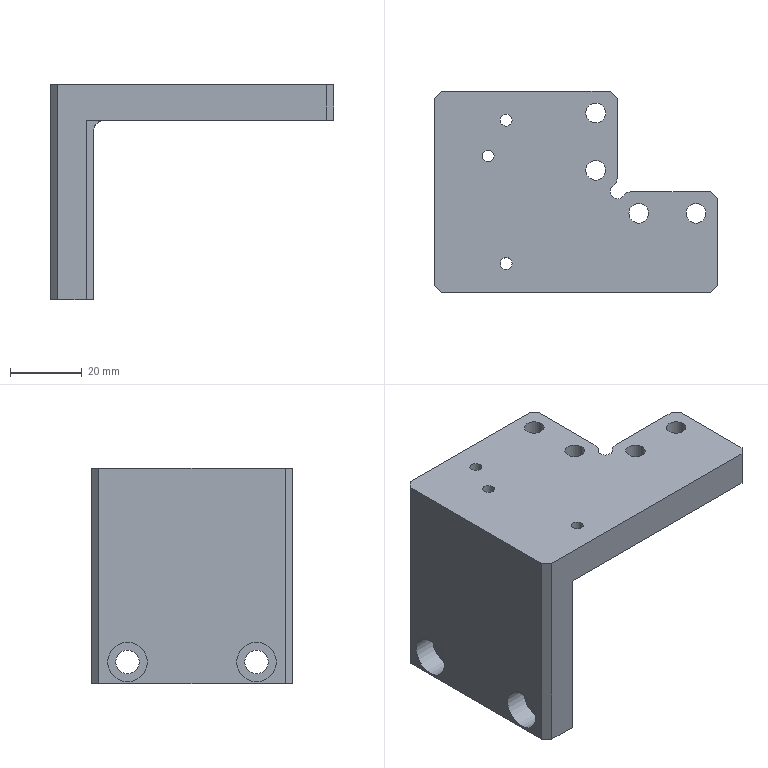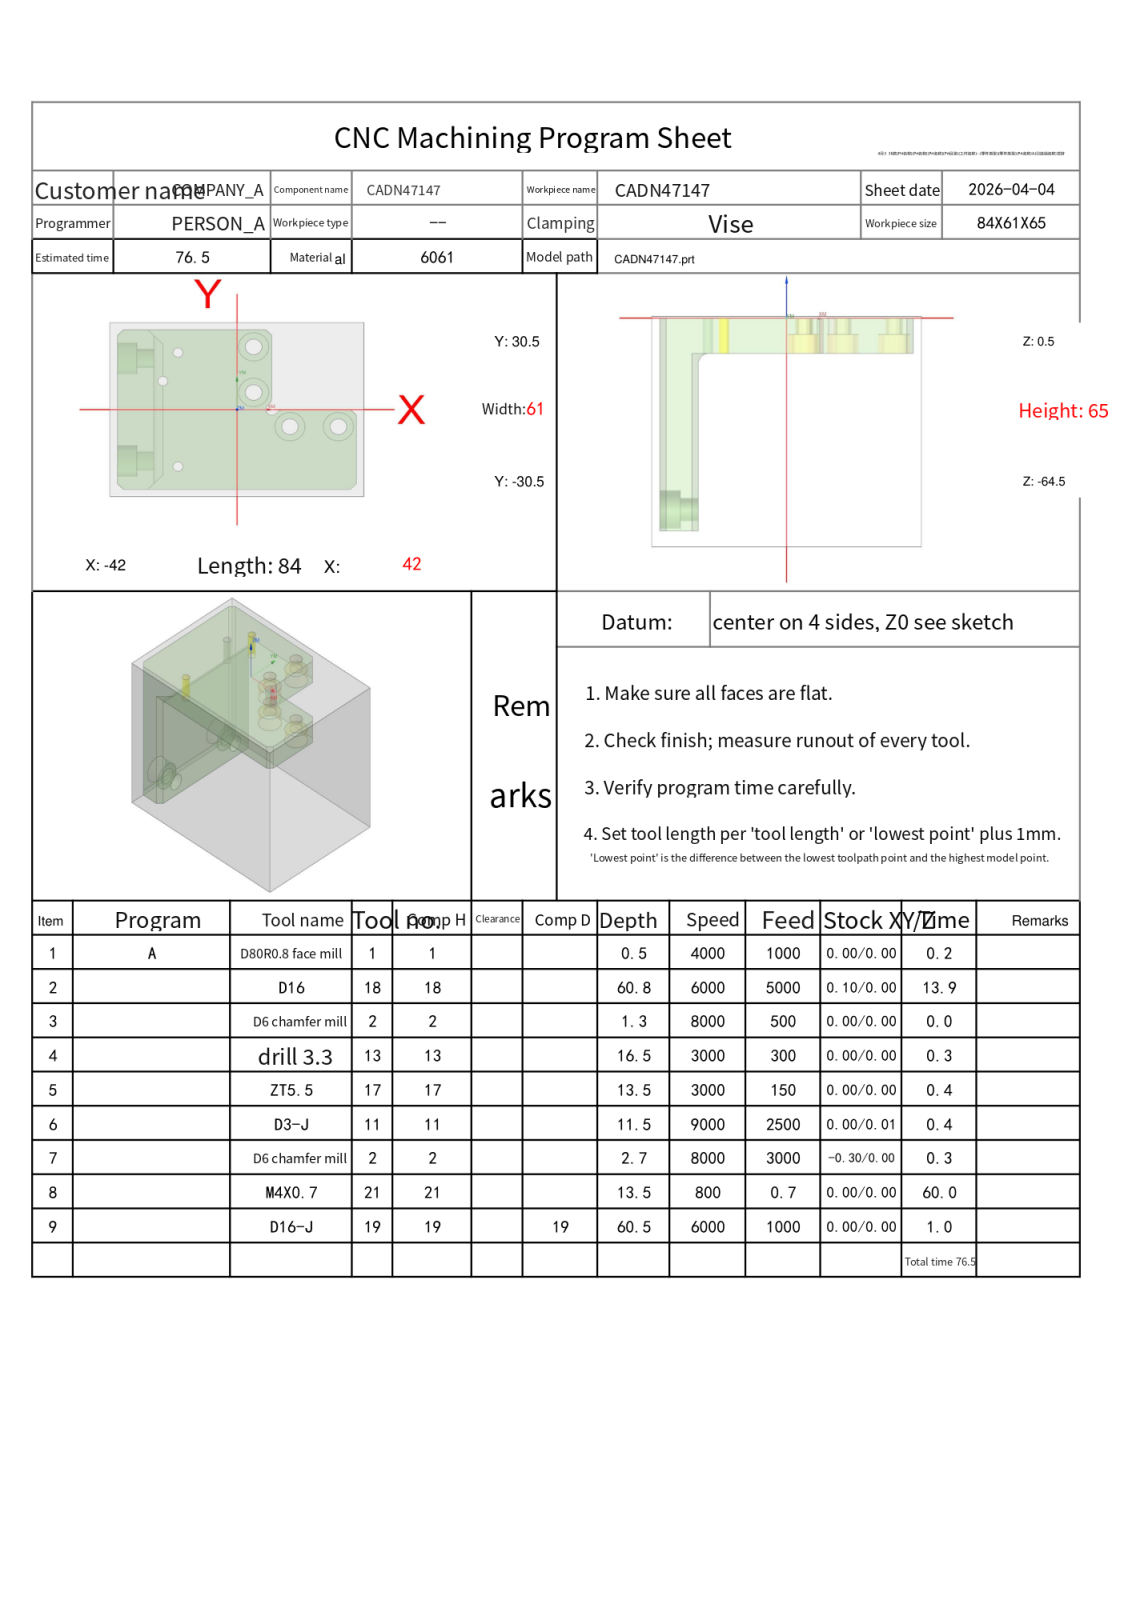NC program | NX | posted by the shop | part box 79 x 56 x 60 mm
Lines 35 to 1262 of 9053:
N2 T18 M06
(D16  D=16. R=0. H=18 ce=0.50 di=0.10)
G00 G90 G54 X61.191 Y31.1 M03 S6000
G43 H18 Z10.5
M08
Z.702
G01 Z-.498 F4000.
X54.
G03 X42.8 Y19.9 I0.0 J-11.2
G01 Y9.341
G02 X45.094 Y7.594 I-5.3 J-9.341
G01 X47.094 Y5.594
G02 X50. Y.258 I-7.594 J-7.594
G01 Y-7.414
X48.
Y-2.
G03 X45.51 Y4.01 I-8.5 J0.0
G01 X43.51 Y6.01
G03 X37.5 Y8.5 I-6.01 J-6.01
G01 X20.
Y26.
G03 X17.51 Y32.01 I-8.5 J0.0
G01 X15.51 Y34.01
G03 X9.5 Y36.5 I-6.01 J-6.01
G01 X-2.314
X-2.27 Y38.5
X11.758
G02 X17.094 Y35.594 I-2.258 J-10.5
G01 X19.094 Y33.594
G02 X20.841 Y31.3 I-7.594 J-7.594
G01 X42.
G02 X42.8 Y30.5 I0.0 J-.8
G01 Y11.9
G02 X41.2 Y10.3 I-1.6 J0.0
X40.385 Y10.523 I0.0 J1.6
G01 X32.009 Y15.477
G03 X31.195 Y15.7 I-.814 J-1.377
G01 X28.797
G02 X27.2 Y17.297 I.003 J1.6
G01 Y22.503
G02 X28.797 Y24.1 I1.6 J-.003
G01 X34.003
G02 X35.6 Y22.503 I-.003 J-1.6
G01 Y17.297
G02 X35.364 Y16.463 I-1.6 J.003
X35.04 Y16.084 I-1.364 J.837
G03 X33.099 Y12.263 I3.641 J-4.254
G01 X61.2
Z.702
G00 Z3.
G01 X61.191 Y31.1 F6000.
G00 Z.203
G01 Z-.997 F4000.
X54.
G03 X42.8 Y19.9 I0.0 J-11.2
G01 Y9.341
G02 X45.094 Y7.594 I-5.3 J-9.341
G01 X47.094 Y5.594
G02 X50. Y.258 I-7.594 J-7.594
G01 Y-7.414
X48.
Y-2.
G03 X45.51 Y4.01 I-8.5 J0.0
G01 X43.51 Y6.01
G03 X37.5 Y8.5 I-6.01 J-6.01
G01 X20.
Y10.74
Y26.
G03 X17.51 Y32.01 I-8.5 J0.0
G01 X15.51 Y34.01
G03 X9.5 Y36.5 I-6.01 J-6.01
G01 X-2.314
X-2.27 Y38.5
X11.758
G02 X17.094 Y35.594 I-2.258 J-10.5
G01 X19.094 Y33.594
G02 X20.841 Y31.3 I-7.594 J-7.594
G01 X42.
G02 X42.8 Y30.5 I0.0 J-.8
G01 Y11.9
G02 X41.2 Y10.3 I-1.6 J0.0
X40.385 Y10.523 I0.0 J1.6
G01 X32.009 Y15.477
G03 X31.195 Y15.7 I-.814 J-1.377
G01 X28.798
G02 X27.2 Y17.298 I.002 J1.6
G01 Y22.502
G02 X28.798 Y24.1 I1.6 J-.002
G01 X34.002
G02 X35.6 Y22.502 I-.002 J-1.6
G01 Y17.298
G02 X35.364 Y16.463 I-1.6 J.002
X35.04 Y16.084 I-1.364 J.837
G03 X33.099 Y12.263 I3.641 J-4.254
G01 X61.2
Z.203
G00 Z2.502
G01 X61.191 Y31.1 F6000.
G00 Z-.295
G01 Z-1.495 F4000.
X54.
G03 X42.8 Y19.9 I0.0 J-11.2
G01 Y9.341
G02 X45.094 Y7.594 I-5.3 J-9.341
G01 X47.094 Y5.594
G02 X50. Y.258 I-7.594 J-7.594
G01 Y-7.414
X48.
Y-2.
G03 X45.51 Y4.01 I-8.5 J0.0
G01 X43.51 Y6.01
G03 X37.5 Y8.5 I-6.01 J-6.01
G01 X20.
Y26.
G03 X17.51 Y32.01 I-8.5 J0.0
G01 X15.51 Y34.01
G03 X9.5 Y36.5 I-6.01 J-6.01
G01 X-2.314
X-2.27 Y38.5
X11.758
G02 X17.094 Y35.594 I-2.258 J-10.5
G01 X19.094 Y33.594
G02 X20.841 Y31.3 I-7.594 J-7.594
G01 X42.
G02 X42.8 Y30.5 I0.0 J-.8
G01 Y11.9
G02 X41.2 Y10.3 I-1.6 J0.0
X40.385 Y10.523 I0.0 J1.6
G01 X32.009 Y15.477
G03 X31.195 Y15.7 I-.814 J-1.377
G01 X28.797
G02 X27.2 Y17.297 I.003 J1.6
G01 Y22.503
G02 X28.797 Y24.1 I1.6 J-.003
G01 X34.003
G02 X35.6 Y22.503 I-.003 J-1.6
G01 Y17.297
G02 X35.364 Y16.463 I-1.6 J.003
X35.04 Y16.084 I-1.364 J.837
G03 X33.099 Y12.263 I3.641 J-4.254
G01 X61.2
Z-.295
G00 Z2.003
G01 X61.191 Y31.1 F6000.
G00 Z-.793
G01 Z-1.993 F4000.
X54.
G03 X42.8 Y19.9 I0.0 J-11.2
G01 Y9.341
G02 X45.094 Y7.594 I-5.3 J-9.341
G01 X47.094 Y5.594
G02 X50. Y.258 I-7.594 J-7.594
G01 Y-7.414
X48.
Y-2.
G03 X45.51 Y4.01 I-8.5 J0.0
G01 X43.51 Y6.01
G03 X37.5 Y8.5 I-6.01 J-6.01
G01 X20.
Y10.74
Y26.
G03 X17.51 Y32.01 I-8.5 J0.0
G01 X15.51 Y34.01
G03 X9.5 Y36.5 I-6.01 J-6.01
G01 X-2.314
X-2.27 Y38.5
X11.758
G02 X17.094 Y35.594 I-2.258 J-10.5
G01 X19.094 Y33.594
G02 X20.841 Y31.3 I-7.594 J-7.594
G01 X42.
G02 X42.8 Y30.5 I0.0 J-.8
G01 Y11.9
G02 X41.2 Y10.3 I-1.6 J0.0
X40.385 Y10.523 I0.0 J1.6
G01 X32.009 Y15.477
G03 X31.195 Y15.7 I-.814 J-1.377
G01 X28.798
G02 X27.2 Y17.298 I.002 J1.6
G01 Y22.502
G02 X28.798 Y24.1 I1.6 J-.002
G01 X34.002
G02 X35.6 Y22.502 I-.002 J-1.6
G01 Y17.298
G02 X35.364 Y16.463 I-1.6 J.002
X35.04 Y16.084 I-1.364 J.837
G03 X33.099 Y12.263 I3.641 J-4.254
G01 X61.2
Z-.793
G00 Z1.505
G01 X61.191 Y31.1 F6000.
G00 Z-1.292
G01 Z-2.492 F4000.
X54.
G03 X42.8 Y19.9 I0.0 J-11.2
G01 Y9.341
G02 X45.094 Y7.594 I-5.3 J-9.341
G01 X47.094 Y5.594
G02 X50. Y.258 I-7.594 J-7.594
G01 Y-7.414
X48.
Y-2.
G03 X45.51 Y4.01 I-8.5 J0.0
G01 X43.51 Y6.01
G03 X37.5 Y8.5 I-6.01 J-6.01
G01 X20.
Y26.
G03 X17.51 Y32.01 I-8.5 J0.0
G01 X15.51 Y34.01
G03 X9.5 Y36.5 I-6.01 J-6.01
G01 X-2.314
X-2.27 Y38.5
X11.758
G02 X17.094 Y35.594 I-2.258 J-10.5
G01 X19.094 Y33.594
G02 X20.841 Y31.3 I-7.594 J-7.594
G01 X42.
G02 X42.8 Y30.5 I0.0 J-.8
G01 Y11.9
G02 X41.2 Y10.3 I-1.6 J0.0
X40.385 Y10.523 I0.0 J1.6
G01 X32.009 Y15.477
G03 X31.195 Y15.7 I-.814 J-1.377
G01 X28.797
G02 X27.2 Y17.297 I.003 J1.6
G01 Y22.503
G02 X28.797 Y24.1 I1.6 J-.003
G01 X34.003
G02 X35.6 Y22.503 I-.003 J-1.6
G01 Y17.297
G02 X35.364 Y16.463 I-1.6 J.003
X35.04 Y16.084 I-1.364 J.837
G03 X33.099 Y12.263 I3.641 J-4.254
G01 X61.2
Z-1.292
G00 Z1.007
G01 X61.191 Y31.1 F6000.
G00 Z-1.79
G01 Z-2.99 F4000.
X54.
G03 X42.8 Y19.9 I0.0 J-11.2
G01 Y9.341
G02 X45.094 Y7.594 I-5.3 J-9.341
G01 X47.094 Y5.594
G02 X50. Y.258 I-7.594 J-7.594
G01 Y-7.414
X48.
Y-2.
G03 X45.51 Y4.01 I-8.5 J0.0
G01 X43.51 Y6.01
G03 X37.5 Y8.5 I-6.01 J-6.01
G01 X20.
Y10.74
Y26.
G03 X17.51 Y32.01 I-8.5 J0.0
G01 X15.51 Y34.01
G03 X9.5 Y36.5 I-6.01 J-6.01
G01 X-2.314
X-2.27 Y38.5
X11.758
G02 X17.094 Y35.594 I-2.258 J-10.5
G01 X19.094 Y33.594
G02 X20.841 Y31.3 I-7.594 J-7.594
G01 X42.
G02 X42.8 Y30.5 I0.0 J-.8
G01 Y11.9
G02 X41.2 Y10.3 I-1.6 J0.0
X40.385 Y10.523 I0.0 J1.6
G01 X32.009 Y15.477
G03 X31.195 Y15.7 I-.814 J-1.377
G01 X28.798
G02 X27.2 Y17.298 I.002 J1.6
G01 Y22.502
G02 X28.798 Y24.1 I1.6 J-.002
G01 X34.002
G02 X35.6 Y22.502 I-.002 J-1.6
G01 Y17.298
G02 X35.364 Y16.463 I-1.6 J.002
X35.04 Y16.084 I-1.364 J.837
G03 X33.099 Y12.263 I3.641 J-4.254
G01 X61.2
Z-1.79
G00 Z.508
G01 X61.191 Y31.1 F6000.
G00 Z-2.288
G01 Z-3.488 F4000.
X54.
G03 X42.8 Y19.9 I0.0 J-11.2
G01 Y9.341
G02 X45.094 Y7.594 I-5.3 J-9.341
G01 X47.094 Y5.594
G02 X50. Y.258 I-7.594 J-7.594
G01 Y-7.414
X48.
Y-2.
G03 X45.51 Y4.01 I-8.5 J0.0
G01 X43.51 Y6.01
G03 X37.5 Y8.5 I-6.01 J-6.01
G01 X20.
Y26.
G03 X17.51 Y32.01 I-8.5 J0.0
G01 X15.51 Y34.01
G03 X9.5 Y36.5 I-6.01 J-6.01
G01 X-2.314
X-2.27 Y38.5
X11.758
G02 X17.094 Y35.594 I-2.258 J-10.5
G01 X19.094 Y33.594
G02 X20.841 Y31.3 I-7.594 J-7.594
G01 X42.
G02 X42.8 Y30.5 I0.0 J-.8
G01 Y11.9
G02 X41.2 Y10.3 I-1.6 J0.0
X40.385 Y10.523 I0.0 J1.6
G01 X32.009 Y15.477
G03 X31.195 Y15.7 I-.814 J-1.377
G01 X28.797
G02 X27.2 Y17.297 I.003 J1.6
G01 Y22.503
G02 X28.797 Y24.1 I1.6 J-.003
G01 X34.003
G02 X35.6 Y22.503 I-.003 J-1.6
G01 Y17.297
G02 X35.364 Y16.463 I-1.6 J.003
X35.04 Y16.084 I-1.364 J.837
G03 X33.099 Y12.263 I3.641 J-4.254
G01 X61.2
Z-2.288
G00 Z.01
G01 X61.191 Y31.1 F6000.
G00 Z-2.787
G01 Z-3.987 F4000.
X54.
G03 X42.8 Y19.9 I0.0 J-11.2
G01 Y9.341
G02 X45.094 Y7.594 I-5.3 J-9.341
G01 X47.094 Y5.594
G02 X50. Y.258 I-7.594 J-7.594
G01 Y-7.414
X48.
Y-2.
G03 X45.51 Y4.01 I-8.5 J0.0
G01 X43.51 Y6.01
G03 X37.5 Y8.5 I-6.01 J-6.01
G01 X20.
Y10.74
Y26.
G03 X17.51 Y32.01 I-8.5 J0.0
G01 X15.51 Y34.01
G03 X9.5 Y36.5 I-6.01 J-6.01
G01 X-2.314
X-2.27 Y38.5
X11.758
G02 X17.094 Y35.594 I-2.258 J-10.5
G01 X19.094 Y33.594
G02 X20.841 Y31.3 I-7.594 J-7.594
G01 X42.
G02 X42.8 Y30.5 I0.0 J-.8
G01 Y11.9
G02 X41.2 Y10.3 I-1.6 J0.0
X40.385 Y10.523 I0.0 J1.6
G01 X32.009 Y15.477
G03 X31.195 Y15.7 I-.814 J-1.377
G01 X28.798
G02 X27.2 Y17.298 I.002 J1.6
G01 Y22.502
G02 X28.798 Y24.1 I1.6 J-.002
G01 X34.002
G02 X35.6 Y22.502 I-.002 J-1.6
G01 Y17.298
G02 X35.364 Y16.463 I-1.6 J.002
X35.04 Y16.084 I-1.364 J.837
G03 X33.099 Y12.263 I3.641 J-4.254
G01 X61.2
Z-2.787
G00 Z-.488
G01 X61.191 Y31.1 F6000.
G00 Z-3.285
G01 Z-4.485 F4000.
X54.
G03 X42.8 Y19.9 I0.0 J-11.2
G01 Y9.341
G02 X45.094 Y7.594 I-5.3 J-9.341
G01 X47.094 Y5.594
G02 X50. Y.258 I-7.594 J-7.594
G01 Y-7.414
X48.
Y-2.
G03 X45.51 Y4.01 I-8.5 J0.0
G01 X43.51 Y6.01
G03 X37.5 Y8.5 I-6.01 J-6.01
G01 X20.
Y26.
G03 X17.51 Y32.01 I-8.5 J0.0
G01 X15.51 Y34.01
G03 X9.5 Y36.5 I-6.01 J-6.01
G01 X-2.314
X-2.27 Y38.5
X11.758
G02 X17.094 Y35.594 I-2.258 J-10.5
G01 X19.094 Y33.594
G02 X20.841 Y31.3 I-7.594 J-7.594
G01 X42.
G02 X42.8 Y30.5 I0.0 J-.8
G01 Y11.9
G02 X41.2 Y10.3 I-1.6 J0.0
X40.385 Y10.523 I0.0 J1.6
G01 X32.009 Y15.477
G03 X31.195 Y15.7 I-.814 J-1.377
G01 X28.797
G02 X27.2 Y17.297 I.003 J1.6
G01 Y22.503
G02 X28.797 Y24.1 I1.6 J-.003
G01 X34.003
G02 X35.6 Y22.503 I-.003 J-1.6
G01 Y17.297
G02 X35.364 Y16.463 I-1.6 J.003
X35.04 Y16.084 I-1.364 J.837
G03 X33.099 Y12.263 I3.641 J-4.254
G01 X61.2
Z-3.285
G00 Z-.987
G01 X61.191 Y31.1 F6000.
G00 Z-3.783
G01 Z-4.983 F4000.
X54.
G03 X42.8 Y19.9 I0.0 J-11.2
G01 Y9.341
G02 X45.094 Y7.594 I-5.3 J-9.341
G01 X47.094 Y5.594
G02 X50. Y.258 I-7.594 J-7.594
G01 Y-7.414
X48.
Y-2.
G03 X45.51 Y4.01 I-8.5 J0.0
G01 X43.51 Y6.01
G03 X37.5 Y8.5 I-6.01 J-6.01
G01 X20.
Y10.74
Y26.
G03 X17.51 Y32.01 I-8.5 J0.0
G01 X15.51 Y34.01
G03 X9.5 Y36.5 I-6.01 J-6.01
G01 X-2.314
X-2.27 Y38.5
X11.758
G02 X17.094 Y35.594 I-2.258 J-10.5
G01 X19.094 Y33.594
G02 X20.841 Y31.3 I-7.594 J-7.594
G01 X42.
G02 X42.8 Y30.5 I0.0 J-.8
G01 Y11.9
G02 X41.2 Y10.3 I-1.6 J0.0
X40.385 Y10.523 I0.0 J1.6
G01 X32.009 Y15.477
G03 X31.195 Y15.7 I-.814 J-1.377
G01 X28.798
G02 X27.2 Y17.298 I.002 J1.6
G01 Y22.502
G02 X28.798 Y24.1 I1.6 J-.002
G01 X34.002
G02 X35.6 Y22.502 I-.002 J-1.6
G01 Y17.298
G02 X35.364 Y16.463 I-1.6 J.002
X35.04 Y16.084 I-1.364 J.837
G03 X33.099 Y12.263 I3.641 J-4.254
G01 X61.2
Z-3.783
G00 Z-1.485
G01 X61.191 Y31.1 F6000.
G00 Z-4.282
G01 Z-5.482 F4000.
X54.
G03 X42.8 Y19.9 I0.0 J-11.2
G01 Y9.341
G02 X45.094 Y7.594 I-5.3 J-9.341
G01 X47.094 Y5.594
G02 X50. Y.258 I-7.594 J-7.594
G01 Y-7.414
X48.
Y-2.
G03 X45.51 Y4.01 I-8.5 J0.0
G01 X43.51 Y6.01
G03 X37.5 Y8.5 I-6.01 J-6.01
G01 X20.
Y26.
G03 X17.51 Y32.01 I-8.5 J0.0
G01 X15.51 Y34.01
G03 X9.5 Y36.5 I-6.01 J-6.01
G01 X-2.314
X-2.27 Y38.5
X11.758
G02 X17.094 Y35.594 I-2.258 J-10.5
G01 X19.094 Y33.594
G02 X20.841 Y31.3 I-7.594 J-7.594
G01 X42.
G02 X42.8 Y30.5 I0.0 J-.8
G01 Y11.9
G02 X41.2 Y10.3 I-1.6 J0.0
X40.385 Y10.523 I0.0 J1.6
G01 X32.009 Y15.477
G03 X31.195 Y15.7 I-.814 J-1.377
G01 X28.797
G02 X27.2 Y17.297 I.003 J1.6
G01 Y22.503
G02 X28.797 Y24.1 I1.6 J-.003
G01 X34.003
G02 X35.6 Y22.503 I-.003 J-1.6
G01 Y17.297
G02 X35.364 Y16.463 I-1.6 J.003
X35.04 Y16.084 I-1.364 J.837
G03 X33.099 Y12.263 I3.641 J-4.254
G01 X61.2
Z-4.282
G00 Z-1.983
G01 X61.191 Y31.1 F6000.
G00 Z-4.78
G01 Z-5.98 F4000.
X54.
G03 X42.8 Y19.9 I0.0 J-11.2
G01 Y9.341
G02 X45.094 Y7.594 I-5.3 J-9.341
G01 X47.094 Y5.594
G02 X50. Y.258 I-7.594 J-7.594
G01 Y-7.414
X48.
Y-2.
G03 X45.51 Y4.01 I-8.5 J0.0
G01 X43.51 Y6.01
G03 X37.5 Y8.5 I-6.01 J-6.01
G01 X20.
Y10.74
Y26.
G03 X17.51 Y32.01 I-8.5 J0.0
G01 X15.51 Y34.01
G03 X9.5 Y36.5 I-6.01 J-6.01
G01 X-2.314
X-2.27 Y38.5
X11.758
G02 X17.094 Y35.594 I-2.258 J-10.5
G01 X19.094 Y33.594
G02 X20.841 Y31.3 I-7.594 J-7.594
G01 X42.
G02 X42.8 Y30.5 I0.0 J-.8
G01 Y11.9
G02 X41.2 Y10.3 I-1.6 J0.0
X40.385 Y10.523 I0.0 J1.6
G01 X32.009 Y15.477
G03 X31.195 Y15.7 I-.814 J-1.377
G01 X28.798
G02 X27.2 Y17.298 I.002 J1.6
G01 Y22.502
G02 X28.798 Y24.1 I1.6 J-.002
G01 X34.002
G02 X35.6 Y22.502 I-.002 J-1.6
G01 Y17.298
G02 X35.364 Y16.463 I-1.6 J.002
X35.04 Y16.084 I-1.364 J.837
G03 X33.099 Y12.263 I3.641 J-4.254
G01 X61.2
Z-4.78
G00 Z-2.482
G01 X61.191 Y31.1 F6000.
G00 Z-5.279
G01 Z-6.479 F4000.
X54.
G03 X42.8 Y19.9 I0.0 J-11.2
G01 Y9.341
G02 X45.094 Y7.594 I-5.3 J-9.341
G01 X47.094 Y5.594
G02 X50. Y.258 I-7.594 J-7.594
G01 Y-7.414
X48.
Y-2.
G03 X45.51 Y4.01 I-8.5 J0.0
G01 X43.51 Y6.01
G03 X37.5 Y8.5 I-6.01 J-6.01
G01 X20.
Y26.
G03 X17.51 Y32.01 I-8.5 J0.0
G01 X15.51 Y34.01
G03 X9.5 Y36.5 I-6.01 J-6.01
G01 X-2.314
X-2.27 Y38.5
X11.758
G02 X17.094 Y35.594 I-2.258 J-10.5
G01 X19.094 Y33.594
G02 X20.841 Y31.3 I-7.594 J-7.594
G01 X42.
G02 X42.8 Y30.5 I0.0 J-.8
G01 Y11.9
G02 X41.2 Y10.3 I-1.6 J0.0
X40.385 Y10.523 I0.0 J1.6
G01 X32.009 Y15.477
G03 X31.195 Y15.7 I-.814 J-1.377
G01 X28.797
G02 X27.2 Y17.297 I.003 J1.6
G01 Y22.503
G02 X28.797 Y24.1 I1.6 J-.003
G01 X34.003
G02 X35.6 Y22.503 I-.003 J-1.6
G01 Y17.297
G02 X35.364 Y16.463 I-1.6 J.003
X35.04 Y16.084 I-1.364 J.837
G03 X33.099 Y12.263 I3.641 J-4.254
G01 X61.2
Z-5.279
G00 Z-2.98
G01 X61.191 Y31.1 F6000.
G00 Z-5.777
G01 Z-6.977 F4000.
X54.
G03 X42.8 Y19.9 I0.0 J-11.2
G01 Y9.341
G02 X45.094 Y7.594 I-5.3 J-9.341
G01 X47.094 Y5.594
G02 X50. Y.258 I-7.594 J-7.594
G01 Y-7.414
X48.
Y-2.
G03 X45.51 Y4.01 I-8.5 J0.0
G01 X43.51 Y6.01
G03 X37.5 Y8.5 I-6.01 J-6.01
G01 X20.
Y10.74
Y26.
G03 X17.51 Y32.01 I-8.5 J0.0
G01 X15.51 Y34.01
G03 X9.5 Y36.5 I-6.01 J-6.01
G01 X-2.314
X-2.27 Y38.5
X11.758
G02 X17.094 Y35.594 I-2.258 J-10.5
G01 X19.094 Y33.594
G02 X20.841 Y31.3 I-7.594 J-7.594
G01 X42.
G02 X42.8 Y30.5 I0.0 J-.8
G01 Y11.9
G02 X41.2 Y10.3 I-1.6 J0.0
X40.385 Y10.523 I0.0 J1.6
G01 X32.009 Y15.477
G03 X31.195 Y15.7 I-.814 J-1.377
G01 X28.798
G02 X27.2 Y17.298 I.002 J1.6
G01 Y22.502
G02 X28.798 Y24.1 I1.6 J-.002
G01 X34.002
G02 X35.6 Y22.502 I-.002 J-1.6
G01 Y17.298
G02 X35.364 Y16.463 I-1.6 J.002
X35.04 Y16.084 I-1.364 J.837
G03 X33.099 Y12.263 I3.641 J-4.254
G01 X61.2
Z-5.777
G00 Z-3.479
G01 X61.191 Y31.1 F6000.
G00 Z-6.275
G01 Z-7.475 F4000.
X54.
G03 X42.8 Y19.9 I0.0 J-11.2
G01 Y9.341
G02 X45.094 Y7.594 I-5.3 J-9.341
G01 X47.094 Y5.594
G02 X50. Y.258 I-7.594 J-7.594
G01 Y-7.414
X48.
Y-2.
G03 X45.51 Y4.01 I-8.5 J0.0
G01 X43.51 Y6.01
G03 X37.5 Y8.5 I-6.01 J-6.01
G01 X20.
Y26.
G03 X17.51 Y32.01 I-8.5 J0.0
G01 X15.51 Y34.01
G03 X9.5 Y36.5 I-6.01 J-6.01
G01 X-2.314
X-2.27 Y38.5
X11.758
G02 X17.094 Y35.594 I-2.258 J-10.5
G01 X19.094 Y33.594
G02 X20.841 Y31.3 I-7.594 J-7.594
G01 X42.
G02 X42.8 Y30.5 I0.0 J-.8
G01 Y11.9
G02 X41.2 Y10.3 I-1.6 J0.0
X40.385 Y10.523 I0.0 J1.6
G01 X32.009 Y15.477
G03 X31.195 Y15.7 I-.814 J-1.377
G01 X28.797
G02 X27.2 Y17.297 I.003 J1.6
G01 Y22.503
G02 X28.797 Y24.1 I1.6 J-.003
G01 X34.003
G02 X35.6 Y22.503 I-.003 J-1.6
G01 Y17.297
G02 X35.364 Y16.463 I-1.6 J.003
X35.04 Y16.084 I-1.364 J.837
G03 X33.099 Y12.263 I3.641 J-4.254
G01 X61.2
Z-6.275
G00 Z-3.977
G01 X61.191 Y31.1 F6000.
G00 Z-6.774
G01 Z-7.974 F4000.
X54.
G03 X42.8 Y19.9 I0.0 J-11.2
G01 Y9.341
G02 X45.094 Y7.594 I-5.3 J-9.341
G01 X47.094 Y5.594
G02 X50. Y.258 I-7.594 J-7.594
G01 Y-7.414
X48.
Y-2.
G03 X45.51 Y4.01 I-8.5 J0.0
G01 X43.51 Y6.01
G03 X37.5 Y8.5 I-6.01 J-6.01
G01 X20.
Y10.74
Y26.
G03 X17.51 Y32.01 I-8.5 J0.0
G01 X15.51 Y34.01
G03 X9.5 Y36.5 I-6.01 J-6.01
G01 X-2.314
X-2.27 Y38.5
X11.758
G02 X17.094 Y35.594 I-2.258 J-10.5
G01 X19.094 Y33.594
G02 X20.841 Y31.3 I-7.594 J-7.594
G01 X42.
G02 X42.8 Y30.5 I0.0 J-.8
G01 Y11.9
G02 X41.2 Y10.3 I-1.6 J0.0
X40.385 Y10.523 I0.0 J1.6
G01 X32.009 Y15.477
G03 X31.195 Y15.7 I-.814 J-1.377
G01 X28.798
G02 X27.2 Y17.298 I.002 J1.6
G01 Y22.502
G02 X28.798 Y24.1 I1.6 J-.002
G01 X34.002
G02 X35.6 Y22.502 I-.002 J-1.6
G01 Y17.298
G02 X35.364 Y16.463 I-1.6 J.002
X35.04 Y16.084 I-1.364 J.837
G03 X33.099 Y12.263 I3.641 J-4.254
G01 X61.2
Z-6.774
G00 Z-4.475
G01 X61.191 Y31.1 F6000.
G00 Z-7.272
G01 Z-8.472 F4000.
X54.
G03 X42.8 Y19.9 I0.0 J-11.2
G01 Y9.341
G02 X45.094 Y7.594 I-5.3 J-9.341
G01 X47.094 Y5.594
G02 X50. Y.258 I-7.594 J-7.594
G01 Y-7.414
X48.
Y-2.
G03 X45.51 Y4.01 I-8.5 J0.0
G01 X43.51 Y6.01
G03 X37.5 Y8.5 I-6.01 J-6.01
G01 X20.
Y26.
G03 X17.51 Y32.01 I-8.5 J0.0
G01 X15.51 Y34.01
G03 X9.5 Y36.5 I-6.01 J-6.01
G01 X-2.314
X-2.27 Y38.5
X11.758
G02 X17.094 Y35.594 I-2.258 J-10.5
G01 X19.094 Y33.594
G02 X20.841 Y31.3 I-7.594 J-7.594
G01 X42.
G02 X42.8 Y30.5 I0.0 J-.8
G01 Y11.9
G02 X41.2 Y10.3 I-1.6 J0.0
X40.385 Y10.523 I0.0 J1.6
G01 X32.009 Y15.477
G03 X31.195 Y15.7 I-.814 J-1.377
G01 X28.797
G02 X27.2 Y17.297 I.003 J1.6
G01 Y22.503
G02 X28.797 Y24.1 I1.6 J-.003
G01 X34.003
G02 X35.6 Y22.503 I-.003 J-1.6
G01 Y17.297
G02 X35.364 Y16.463 I-1.6 J.003
X35.04 Y16.084 I-1.364 J.837
G03 X33.099 Y12.263 I3.641 J-4.254
G01 X61.2
Z-7.272
G00 Z-4.974
G01 X61.191 Y31.1 F6000.
G00 Z-7.77
G01 Z-8.97 F4000.
X54.
G03 X42.8 Y19.9 I0.0 J-11.2
G01 Y9.341
G02 X45.094 Y7.594 I-5.3 J-9.341
G01 X47.094 Y5.594
G02 X50. Y.258 I-7.594 J-7.594
G01 Y-7.414
X48.
Y-2.
G03 X45.51 Y4.01 I-8.5 J0.0
G01 X43.51 Y6.01
G03 X37.5 Y8.5 I-6.01 J-6.01
G01 X20.
Y10.74
Y26.
G03 X17.51 Y32.01 I-8.5 J0.0
G01 X15.51 Y34.01
G03 X9.5 Y36.5 I-6.01 J-6.01
G01 X-2.314
X-2.27 Y38.5
X11.758
G02 X17.094 Y35.594 I-2.258 J-10.5
G01 X19.094 Y33.594
G02 X20.841 Y31.3 I-7.594 J-7.594
G01 X42.
G02 X42.8 Y30.5 I0.0 J-.8
G01 Y11.9
G02 X41.2 Y10.3 I-1.6 J0.0
X40.385 Y10.523 I0.0 J1.6
G01 X32.009 Y15.477
G03 X31.195 Y15.7 I-.814 J-1.377
G01 X28.798
G02 X27.2 Y17.298 I.002 J1.6
G01 Y22.502
G02 X28.798 Y24.1 I1.6 J-.002
G01 X34.002
G02 X35.6 Y22.502 I-.002 J-1.6
G01 Y17.298
G02 X35.364 Y16.463 I-1.6 J.002
X35.04 Y16.084 I-1.364 J.837
G03 X33.099 Y12.263 I3.641 J-4.254
G01 X61.2
Z-7.77
G00 Z-5.472
G01 X61.191 Y31.1 F6000.
G00 Z-8.269
G01 Z-9.469 F4000.
X54.
G03 X42.8 Y19.9 I0.0 J-11.2
G01 Y9.341
G02 X45.094 Y7.594 I-5.3 J-9.341
G01 X47.094 Y5.594
G02 X50. Y.258 I-7.594 J-7.594
G01 Y-7.414
X48.
Y-2.
G03 X45.51 Y4.01 I-8.5 J0.0
G01 X43.51 Y6.01
G03 X37.5 Y8.5 I-6.01 J-6.01
G01 X20.
Y26.
G03 X17.51 Y32.01 I-8.5 J0.0
G01 X15.51 Y34.01
G03 X9.5 Y36.5 I-6.01 J-6.01
G01 X-2.314
X-2.27 Y38.5
X11.758
G02 X17.094 Y35.594 I-2.258 J-10.5
G01 X19.094 Y33.594
G02 X20.841 Y31.3 I-7.594 J-7.594
G01 X42.
G02 X42.8 Y30.5 I0.0 J-.8
G01 Y11.9
G02 X41.2 Y10.3 I-1.6 J0.0
X40.385 Y10.523 I0.0 J1.6
G01 X32.009 Y15.477
G03 X31.195 Y15.7 I-.814 J-1.377
G01 X28.797
G02 X27.2 Y17.297 I.003 J1.6
G01 Y22.503
G02 X28.797 Y24.1 I1.6 J-.003
G01 X34.003
G02 X35.6 Y22.503 I-.003 J-1.6
G01 Y17.297
G02 X35.364 Y16.463 I-1.6 J.003
X35.04 Y16.084 I-1.364 J.837
G03 X33.099 Y12.263 I3.641 J-4.254
G01 X61.2
Z-8.269
G00 Z-5.97
G01 X61.191 Y31.1 F6000.
G00 Z-8.767
G01 Z-9.967 F4000.
X54.
G03 X42.8 Y19.9 I0.0 J-11.2
G01 Y9.341
G02 X45.094 Y7.594 I-5.3 J-9.341
G01 X47.094 Y5.594
G02 X50. Y.258 I-7.594 J-7.594
G01 Y-7.414
X48.
Y-2.
G03 X45.51 Y4.01 I-8.5 J0.0
G01 X43.51 Y6.01
G03 X37.5 Y8.5 I-6.01 J-6.01
G01 X20.
Y10.74
Y26.
G03 X17.51 Y32.01 I-8.5 J0.0
G01 X15.51 Y34.01
G03 X9.5 Y36.5 I-6.01 J-6.01
G01 X-2.314
X-2.27 Y38.5
X11.758
G02 X17.094 Y35.594 I-2.258 J-10.5
G01 X19.094 Y33.594
G02 X20.841 Y31.3 I-7.594 J-7.594
G01 X42.
G02 X42.8 Y30.5 I0.0 J-.8
G01 Y11.9
G02 X41.2 Y10.3 I-1.6 J0.0
X40.385 Y10.523 I0.0 J1.6
G01 X32.009 Y15.477
G03 X31.195 Y15.7 I-.814 J-1.377
G01 X28.798
G02 X27.2 Y17.298 I.002 J1.6
G01 Y22.502
G02 X28.798 Y24.1 I1.6 J-.002
G01 X34.002
G02 X35.6 Y22.502 I-.002 J-1.6
G01 Y17.298
G02 X35.364 Y16.463 I-1.6 J.002
X35.04 Y16.084 I-1.364 J.837
G03 X33.099 Y12.263 I3.641 J-4.254
G01 X61.2
Z-8.767
G00 Z-6.469
G01 X61.191 Y31.1 F6000.
G00 Z-9.265
G01 Z-10.465 F4000.
X54.
G03 X42.8 Y19.9 I0.0 J-11.2
G01 Y9.341
G02 X45.095 Y7.594 I-5.3 J-9.341
G01 X47.094 Y5.594
G02 X50. Y.258 I-7.594 J-7.594
G01 Y-7.414
X48.
Y-2.
G03 X45.51 Y4.01 I-8.5 J0.0
G01 X43.51 Y6.01
G03 X37.5 Y8.5 I-6.01 J-6.01
G01 X20.
Y26.
G03 X17.51 Y32.01 I-8.5 J0.0
G01 X15.51 Y34.01
G03 X9.5 Y36.5 I-6.01 J-6.01
G01 X-2.314
X-2.27 Y38.5
X11.758
G02 X17.094 Y35.594 I-2.258 J-10.5
G01 X19.094 Y33.594
G02 X20.841 Y31.3 I-7.594 J-7.594
G01 X42.
G02 X42.8 Y30.5 I0.0 J-.8
G01 Y11.9
G02 X41.2 Y10.3 I-1.6 J0.0
X40.385 Y10.523 I0.0 J1.6
G01 X32.009 Y15.477
G03 X31.195 Y15.7 I-.814 J-1.377
G01 X28.797
G02 X27.2 Y17.297 I.003 J1.6
G01 Y22.503
G02 X28.797 Y24.1 I1.6 J-.003
G01 X34.003
G02 X35.6 Y22.503 I-.003 J-1.6
G01 Y17.297
G02 X35.364 Y16.463 I-1.6 J.003
X35.04 Y16.084 I-1.364 J.837
G03 X33.099 Y12.263 I3.641 J-4.254
G01 X61.2
Z-9.265
G00 Z-6.967
G01 X61.191 Y31.1 F6000.
G00 Z-9.764
G01 Z-10.964 F4000.
X54.
G03 X42.8 Y19.9 I0.0 J-11.2
G01 Y9.341
G02 X45.094 Y7.594 I-5.3 J-9.341
G01 X47.094 Y5.594
G02 X50. Y.258 I-7.594 J-7.594
G01 Y-7.414
X48.
Y-2.
G03 X45.51 Y4.01 I-8.5 J0.0
G01 X43.51 Y6.01
G03 X37.5 Y8.5 I-6.01 J-6.01
G01 X20.
Y26.
G03 X17.51 Y32.01 I-8.5 J0.0
G01 X15.51 Y34.01
G03 X9.5 Y36.5 I-6.01 J-6.01
G01 X-2.314
X-2.27 Y38.5
X11.758
G02 X17.094 Y35.594 I-2.258 J-10.5
G01 X19.094 Y33.594
G02 X20.841 Y31.3 I-7.594 J-7.594
G01 X42.
G02 X42.8 Y30.5 I0.0 J-.8
G01 Y11.9
G02 X41.2 Y10.3 I-1.6 J0.0
X40.385 Y10.523 I0.0 J1.6
G01 X32.009 Y15.477
G03 X31.195 Y15.7 I-.814 J-1.377
G01 X28.798
G02 X27.2 Y17.298 I.002 J1.6
G01 Y22.502
G02 X28.798 Y24.1 I1.6 J-.002
G01 X34.002
G02 X35.6 Y22.502 I-.002 J-1.6
G01 Y17.298
G02 X35.364 Y16.463 I-1.6 J.002
X35.04 Y16.084 I-1.364 J.837
G03 X33.099 Y12.263 I3.641 J-4.254
G01 X61.2
Z-9.764
G00 Z-7.465
G01 X61.191 Y31.1 F6000.
G00 Z-10.262
G01 Z-11.462 F4000.
X54.
G03 X42.8 Y19.9 I0.0 J-11.2
G01 Y9.341
G02 X45.094 Y7.594 I-5.3 J-9.341
G01 X47.094 Y5.594
G02 X50. Y.258 I-7.594 J-7.594
G01 Y-7.414
X48.
Y-2.
G03 X45.51 Y4.01 I-8.5 J0.0
G01 X43.51 Y6.01
G03 X37.5 Y8.5 I-6.01 J-6.01
G01 X20.
Y26.
G03 X17.51 Y32.01 I-8.5 J0.0
G01 X15.51 Y34.01
G03 X9.5 Y36.5 I-6.01 J-6.01
G01 X-2.314
X-2.27 Y38.5
X11.758
G02 X17.094 Y35.594 I-2.258 J-10.5
G01 X19.094 Y33.594
G02 X20.841 Y31.3 I-7.594 J-7.594
G01 X42.
G02 X42.8 Y30.5 I0.0 J-.8
G01 Y11.9
G02 X41.2 Y10.3 I-1.6 J0.0
X40.385 Y10.523 I0.0 J1.6
G01 X32.009 Y15.477
G03 X31.195 Y15.7 I-.814 J-1.377
G01 X28.797
G02 X27.2 Y17.297 I.003 J1.6
G01 Y22.503
G02 X28.797 Y24.1 I1.6 J-.003
G01 X34.003
G02 X35.6 Y22.503 I-.003 J-1.6
G01 Y17.297
G02 X35.364 Y16.463 I-1.6 J.003
X35.04 Y16.084 I-1.364 J.837
G03 X33.099 Y12.263 I3.641 J-4.254
G01 X61.2
Z-10.262
G00 Z-7.964
G01 X61.191 Y31.1 F6000.
G00 Z-10.76
G01 Z-11.96 F4000.
X54.
G03 X42.8 Y19.9 I0.0 J-11.2
G01 Y9.341
G02 X45.094 Y7.594 I-5.3 J-9.341
G01 X47.094 Y5.594
G02 X50. Y.258 I-7.594 J-7.594
G01 Y-7.414
X48.
Y-2.
G03 X45.51 Y4.01 I-8.5 J0.0
G01 X43.51 Y6.01
G03 X37.5 Y8.5 I-6.01 J-6.01
G01 X20.
Y26.
G03 X17.51 Y32.01 I-8.5 J0.0
G01 X15.51 Y34.01
G03 X9.5 Y36.5 I-6.01 J-6.01
G01 X-2.314
X-2.27 Y38.5
X11.758
G02 X17.094 Y35.594 I-2.258 J-10.5
G01 X19.094 Y33.594
G02 X20.841 Y31.3 I-7.594 J-7.594
G01 X42.
G02 X42.8 Y30.5 I0.0 J-.8
G01 Y11.9
G02 X41.2 Y10.3 I-1.6 J0.0
X40.385 Y10.523 I0.0 J1.6
G01 X32.009 Y15.477
G03 X31.195 Y15.7 I-.814 J-1.377
G01 X28.798
G02 X27.2 Y17.298 I.002 J1.6
G01 Y22.502
G02 X28.798 Y24.1 I1.6 J-.002
G01 X34.002
G02 X35.6 Y22.502 I-.002 J-1.6
G01 Y17.298
G02 X35.364 Y16.463 I-1.6 J.002
X35.04 Y16.084 I-1.364 J.837
G03 X33.099 Y12.263 I3.641 J-4.254
G01 X61.2
Z-10.76
G00 Z-8.462
G01 X61.191 Y31.1 F6000.
G00 Z-11.259
G01 Z-12.459 F4000.
X54.
G03 X42.8 Y19.9 I0.0 J-11.2
G01 Y9.341
G02 X45.094 Y7.594 I-5.3 J-9.341
G01 X47.094 Y5.594
G02 X50. Y.258 I-7.594 J-7.594
G01 Y-7.414
X48.
Y-2.
G03 X45.51 Y4.01 I-8.5 J0.0
G01 X43.51 Y6.01
G03 X37.5 Y8.5 I-6.01 J-6.01
G01 X20.
Y26.
G03 X17.51 Y32.01 I-8.5 J0.0
G01 X15.51 Y34.01
G03 X9.5 Y36.5 I-6.01 J-6.01
G01 X-2.314
X-2.27 Y38.5
X11.758
G02 X17.094 Y35.594 I-2.258 J-10.5
G01 X19.094 Y33.594
G02 X20.841 Y31.3 I-7.594 J-7.594
G01 X42.
G02 X42.8 Y30.5 I0.0 J-.8
G01 Y11.9
G02 X41.2 Y10.3 I-1.6 J0.0
X40.385 Y10.523 I0.0 J1.6
G01 X32.009 Y15.477
G03 X31.195 Y15.7 I-.814 J-1.377
G01 X28.797
G02 X27.2 Y17.297 I.003 J1.6
G01 Y22.503
G02 X28.797 Y24.1 I1.6 J-.003
G01 X34.003
G02 X35.6 Y22.503 I-.003 J-1.6
G01 Y17.297
G02 X35.364 Y16.463 I-1.6 J.003
X35.04 Y16.084 I-1.364 J.837
G03 X33.099 Y12.263 I3.641 J-4.254
G01 X61.2
Z-11.259
G00 Z-8.96
G01 X61.191 Y31.1 F6000.
G00 Z-11.757
G01 Z-12.957 F4000.
X54.
G03 X42.8 Y19.9 I0.0 J-11.2
G01 Y9.341
G02 X45.094 Y7.594 I-5.3 J-9.341
G01 X47.094 Y5.594
G02 X50. Y.258 I-7.594 J-7.594
G01 Y-7.414
X48.
Y-2.
G03 X45.51 Y4.01 I-8.5 J0.0
G01 X43.51 Y6.01
G03 X37.5 Y8.5 I-6.01 J-6.01
G01 X20.
Y26.
G03 X17.51 Y32.01 I-8.5 J0.0
G01 X15.51 Y34.01
G03 X9.5 Y36.5 I-6.01 J-6.01
G01 X-2.314
X-2.27 Y38.5
X11.758
G02 X17.094 Y35.594 I-2.258 J-10.5
G01 X19.094 Y33.594
G02 X20.841 Y31.3 I-7.594 J-7.594
G01 X42.
G02 X42.8 Y30.5 I0.0 J-.8
G01 Y11.9
G02 X41.2 Y10.3 I-1.6 J0.0
X40.385 Y10.523 I0.0 J1.6
G01 X32.009 Y15.477
G03 X31.195 Y15.7 I-.814 J-1.377
G01 X28.798
G02 X27.2 Y17.298 I.002 J1.6
G01 Y22.502
G02 X28.798 Y24.1 I1.6 J-.002
G01 X34.002
G02 X35.6 Y22.502 I-.002 J-1.6
G01 Y17.298
G02 X35.364 Y16.463 I-1.6 J.002
X35.04 Y16.084 I-1.364 J.837
G03 X33.099 Y12.263 I3.641 J-4.254
G01 X61.2
Z-11.757
G00 Z-9.459
G01 X61.191 Y31.1 F6000.
G00 Z-12.255
G01 Z-13.455 F4000.
X54.
G03 X42.8 Y19.9 I0.0 J-11.2
G01 Y9.341
G02 X45.094 Y7.594 I-5.3 J-9.341
G01 X47.094 Y5.594
G02 X50. Y.258 I-7.594 J-7.594
G01 Y-7.414
X48.
Y-2.
G03 X45.51 Y4.01 I-8.5 J0.0
G01 X43.51 Y6.01
G03 X37.5 Y8.5 I-6.01 J-6.01
G01 X20.
Y26.
G03 X17.51 Y32.01 I-8.5 J0.0